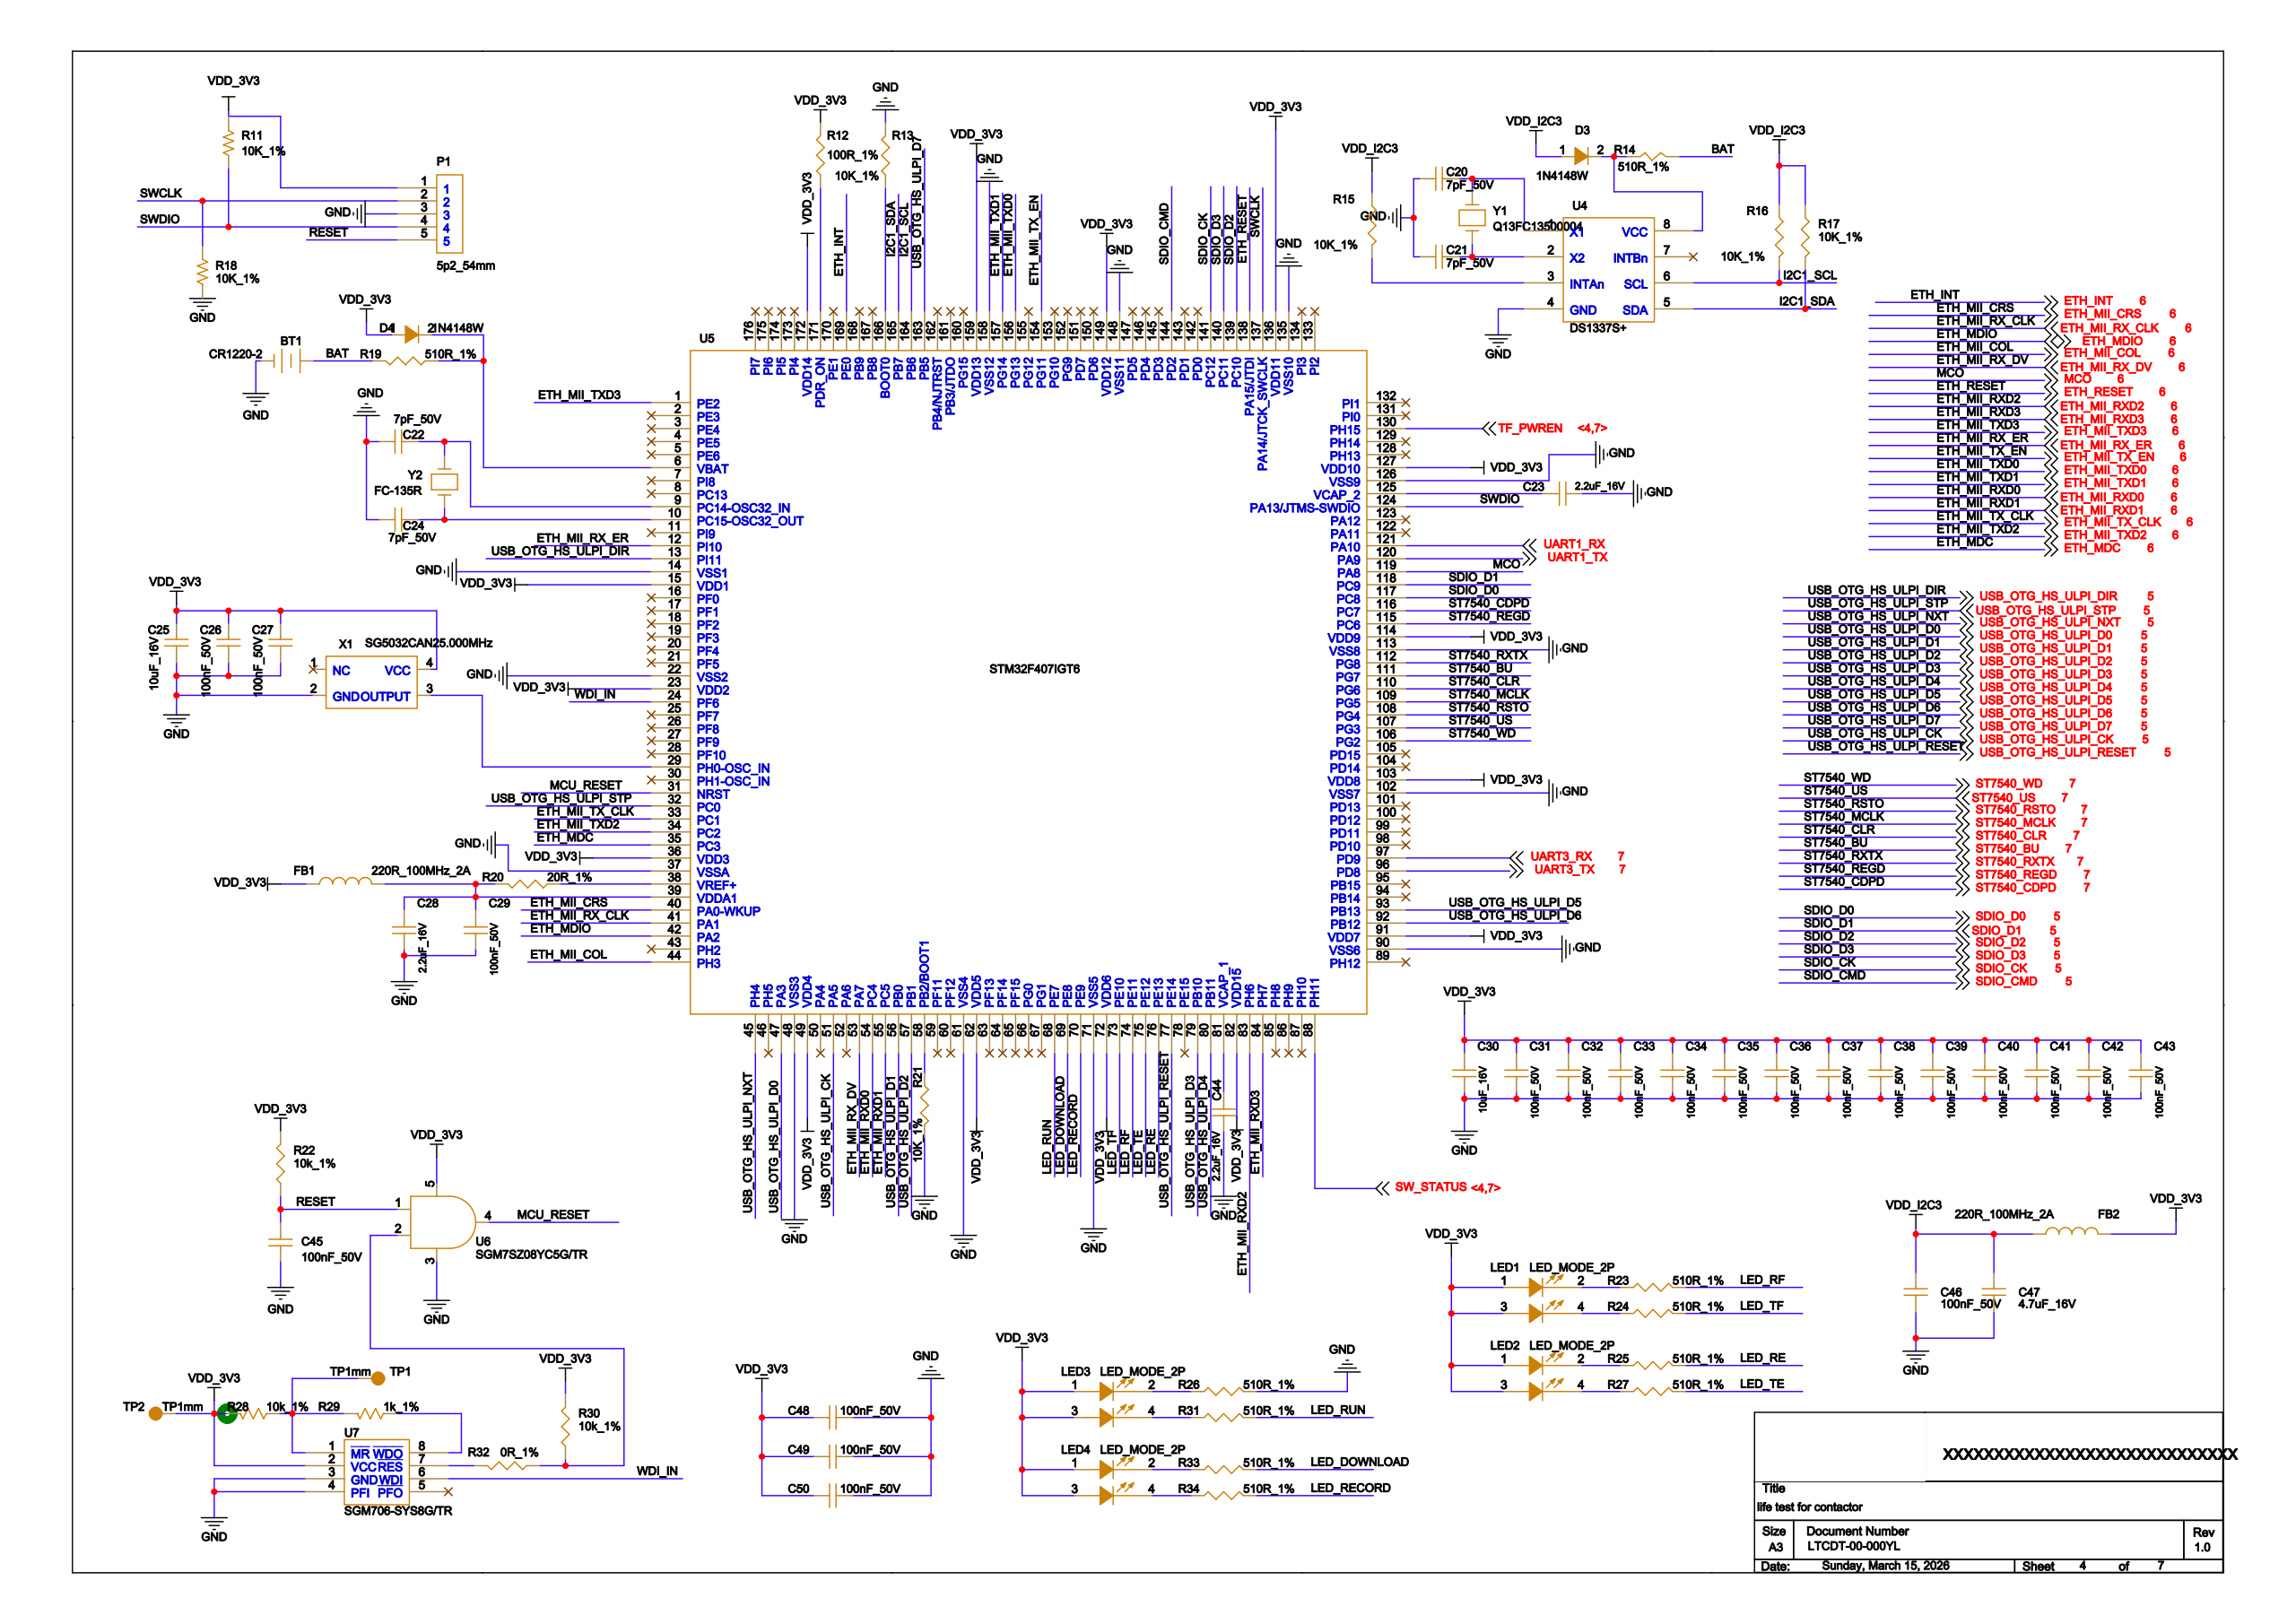Circuit board | Cadence Allegro | 260 parts | 211 nets | one sheet of the schematic
Parts on this sheet (reference | value | footprint):
BT1 | CON_BATTERY_CR2032
C20 | 0603-C
C21 | 0603-C
C22 | 0603-C
C23 | 0603-C
C24 | 0603-C
C44 | 0603-C
C45 | 0603-C
C46 | 0603-C
C47 | 0603-C
C48 | 0603-C
C49 | 0603-C
C50 | 0603-C
D3 | SOD-123
FB1 | 0603-L
FB2 | 0603-L
LED1 | LED-TH_A694B2SYGS530-E2
LED2 | LED-TH_A694B2SYGS530-E2
LED3 | LED-TH_A694B2SYGS530-E2
LED4 | LED-TH_A694B2SYGS530-E2
P1 | 5P2_54MM
R11 | 0603-R
R12 | 0603-R
R13 | 0603-R
R14 | 0603-R
R15 | 0603-R
R16 | 0603-R
R17 | 0603-R
R18 | 0603-R
R19 | 0603-R
R20 | 0603-R
R21 | 0603-R
R22 | 0603-R
R23 | 0603-R
R24 | 0603-R
R25 | 0603-R
R26 | 0603-R
R27 | 0603-R
R28 | 0603-R
R29 | 0603-R
R30 | 0603-R
R31 | 0603-R
R32 | 0603-R
R33 | 0603-R
R34 | 0603-R
TP1 | TP_SMD1MMCIRCLE
TP2 | TP_SMD1MMCIRCLE
U4 | 21-0041B_8
U5 | LQFP176
U6 | SOT-23-5-0_95-H1_45
U7 | SOIC8-1_27-3_98-1_75
Y1 | X2-3_2X1_5-FC-135R
Y2 | X2-3_2X1_5-FC-135R
Nets of these parts (net: part-pin ...):
GND: BT1-2 C20-1 C21-1 C22-1 C23-1 C24-1 C44-1 C45-1 C46-2 C47-2 C48-2 C49-2 C50-2 P1-3 R13-1 R18-1 R21-1 R26-2 U4-4 U6-3 U7-3 U7-4 U5-14 U5-22 U5-37 U5-48 U5-61 U5-71 U5-90 U5-102 U5-113 U5-126 U5-135 U5-148 U5-158
TF_PWREN: U5-130
BAT: BT1-1 R14-2 R19-1
VDD_3V3: C48-1 C49-1 C50-1 FB1-2 FB2-2 LED1-1 LED1-3 LED2-1 LED2-3 LED3-1 LED3-3 LED4-1 LED4-3 P1-1 R11-1 R12-1 R22-2 R28-2 R30-2 TP2-1 U6-5 U7-2 U5-15 U5-23 U5-36 U5-49 U5-62 U5-72 U5-82 U5-91 U5-103 U5-114 U5-127 U5-136 U5-149 U5-159 U5-172
N17276843: C20-2 U4-1 Y1-2
N17276918: C21-2 U4-2 Y1-1
N17213940: C22-2 Y2-1 U5-9
N17213962: C24-2 Y2-2 U5-10
N16993200: C23-2 U5-125
N16993359: FB1-1 R20-1 U5-39
N16993423: C44-2 U5-81
RESET: C45-2 P1-5 R22-1 U6-1
VDD_I2C3: C46-1 C47-1 D3-1 FB2-1 R15-1 R16-1 R17-1
N17276825: D3-2 R14-1 U4-8
N17215836: R19-2 U5-6
SW_STATUS: U5-88
N17270446: LED1-2 R23-1
N17270462: LED1-4 R24-1
N17270489: LED2-2 R25-1
N17270504: LED2-4 R27-1
N17269715: LED3-2 R26-1
N17269736: LED3-4 R31-1
N17269767: LED4-2 R33-1
N17269786: LED4-4 R34-1
SWCLK: P1-2 R18-2 U5-137
SWDIO: P1-4 R11-2 U5-124
N16992347: R13-2 U5-166
N16993778: R21-2 U5-58
SDIO_D3: U5-140
SDIO_D2: U5-139
SDIO_D0: U5-117
SDIO_D1: U5-118
SDIO_CMD: U5-144
N16993902: R12-2 U5-171
N17276920: R15-2 U4-3
I2C1_SCL: R16-2 U4-6 U5-164
I2C1_SDA: R17-2 U4-5 U5-165
LED_RF: R23-2 U5-74
LED_TF: R24-2 U5-73
LED_RE: R25-2 U5-76
LED_TE: R27-2 U5-75
LED_RUN: R31-2 U5-68
LED_DOWNLOAD: R33-2 U5-69
LED_RECORD: R34-2 U5-70
N16993405: R20-2 U5-38
N17265345: R28-1 R29-2 TP1-1 U7-1
N17265388: R29-1 U7-8
N17265312: R30-1 R32-1 U6-2
N17265428: R32-2 U7-7
USB_OTG_HS_ULPI_RESET: U5-77
USB_OTG_HS_ULPI_CK: U5-51
SDIO_CK: U5-141
ETH_RESET: U5-138
ETH_INT: U5-169
ETH_MDIO: U5-42
MCO: U5-119
ETH_MII_RXD0: U5-54
ETH_MII_RXD1: U5-55
ETH_MII_RXD2: U5-83
ETH_MII_RXD3: U5-84
ETH_MII_RX_DV: U5-53
ETH_MII_CRS: U5-40
ETH_MII_RX_ER: U5-12
ETH_MII_COL: U5-44
ETH_MII_TXD0: U5-156
ETH_MII_TXD1: U5-157
ETH_MII_TXD2: U5-34
ETH_MII_TXD3: U5-1
ETH_MII_TX_CLK: U5-33
ETH_MII_TX_EN: U5-154
USB_OTG_HS_ULPI_D0: U5-47
USB_OTG_HS_ULPI_D1: U5-56
USB_OTG_HS_ULPI_D2: U5-57
USB_OTG_HS_ULPI_D3: U5-79
USB_OTG_HS_ULPI_D4: U5-80
USB_OTG_HS_ULPI_D5: U5-93
USB_OTG_HS_ULPI_D6: U5-92
USB_OTG_HS_ULPI_D7: U5-163
USB_OTG_HS_ULPI_DIR: U5-13
USB_OTG_HS_ULPI_NXT: U5-45
USB_OTG_HS_ULPI_STP: U5-32
UART1_RX: U5-121
UART1_TX: U5-120
ETH_MDC: U5-35
ETH_MII_RX_CLK: U5-41
ST7540_BU: U5-111
ST7540_CDPD: U5-116
ST7540_CLR: U5-110
ST7540_MCLK: U5-109
ST7540_REGD: U5-115
ST7540_RSTO: U5-108
UART3_RX: U5-97
ST7540_RXTX: U5-112
UART3_TX: U5-96
ST7540_US: U5-107
ST7540_WD: U5-106
MCU_RESET: U6-4 U5-31
WDI_IN: U7-6 U5-24